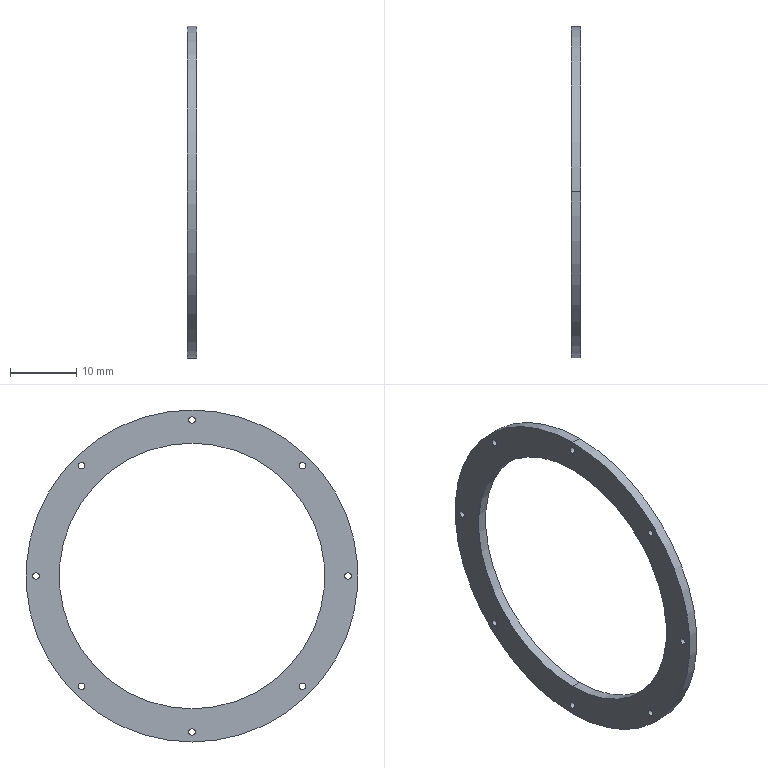Part | SolidWorks | features SavedExtBody 1 | 1 solid | 22 faces | box 1.5 x 50 x 50 mm | volume 1051 mm3 | cylinder 20 | plane 2 | commonest cylinder face diameters 1 x16 40 x2 50 x2
STEP:
#1=CARTESIAN_POINT('',(-88.272,23.5,64.5));
#2=VERTEX_POINT('',#1);
#3=CARTESIAN_POINT('',(-88.272,23.5,65.5));
#4=VERTEX_POINT('',#3);
#5=CARTESIAN_POINT('',(-88.272,23.5,65.));
#6=DIRECTION('',(-1.,0.,0.));
#7=DIRECTION('',(0.,0.,1.));
#8=AXIS2_PLACEMENT_3D('',#5,#6,#7);
#9=CIRCLE('',#8,0.5);
#10=EDGE_CURVE('',#2,#4,#9,.T.);
#11=ORIENTED_EDGE('',*,*,#10,.F.);
#12=CARTESIAN_POINT('',(-89.772,23.5,64.5));
#13=VERTEX_POINT('',#12);
#14=CARTESIAN_POINT('',(-88.272,23.5,64.5));
#15=DIRECTION('',(-1.,0.,0.));
#16=VECTOR('',#15,1000.);
#17=LINE('',#14,#16);
#18=EDGE_CURVE('',#2,#13,#17,.T.);
#19=ORIENTED_EDGE('',*,*,#18,.T.);
#20=CARTESIAN_POINT('',(-89.772,23.5,65.5));
#21=VERTEX_POINT('',#20);
#22=CARTESIAN_POINT('',(-89.772,23.5,65.));
#23=DIRECTION('',(-1.,0.,0.));
#24=DIRECTION('',(0.,0.,1.));
#25=AXIS2_PLACEMENT_3D('',#22,#23,#24);
#26=CIRCLE('',#25,0.5);
#27=EDGE_CURVE('',#13,#21,#26,.T.);
#28=ORIENTED_EDGE('',*,*,#27,.T.);
#29=CARTESIAN_POINT('',(-88.272,23.5,65.5));
#30=DIRECTION('',(-1.,0.,0.));
#31=VECTOR('',#30,1000.);
#32=LINE('',#29,#31);
#33=EDGE_CURVE('',#4,#21,#32,.T.);
#34=ORIENTED_EDGE('',*,*,#33,.F.);
#35=EDGE_LOOP('',(#11,#19,#28,#34));
#36=FACE_OUTER_BOUND('',#35,.T.);
#37=CARTESIAN_POINT('',(-88.272,23.5,65.));
#38=DIRECTION('',(-1.,0.,0.));
#39=DIRECTION('',(0.,0.,1.));
#40=AXIS2_PLACEMENT_3D('',#37,#38,#39);
#41=CYLINDRICAL_SURFACE('',#40,0.5);
#42=ADVANCED_FACE('',(#36),#41,.F.);
#43=CARTESIAN_POINT('',(-88.272,16.617,81.117));
#44=VERTEX_POINT('',#43);
#45=CARTESIAN_POINT('',(-88.272,16.617,82.117));
#46=VERTEX_POINT('',#45);
#47=CARTESIAN_POINT('',(-88.272,16.617,81.617));
#48=DIRECTION('',(-1.,0.,0.));
#49=DIRECTION('',(0.,0.,1.));
#50=AXIS2_PLACEMENT_3D('',#47,#48,#49);
#51=CIRCLE('',#50,0.5);
#52=EDGE_CURVE('',#44,#46,#51,.T.);
#53=ORIENTED_EDGE('',*,*,#52,.F.);
#54=CARTESIAN_POINT('',(-89.772,16.617,81.117));
#55=VERTEX_POINT('',#54);
#56=CARTESIAN_POINT('',(-88.272,16.617,81.117));
#57=DIRECTION('',(-1.,0.,0.));
#58=VECTOR('',#57,1000.);
#59=LINE('',#56,#58);
#60=EDGE_CURVE('',#44,#55,#59,.T.);
#61=ORIENTED_EDGE('',*,*,#60,.T.);
#62=CARTESIAN_POINT('',(-89.772,16.617,82.117));
#63=VERTEX_POINT('',#62);
#64=CARTESIAN_POINT('',(-89.772,16.617,81.617));
#65=DIRECTION('',(-1.,0.,0.));
#66=DIRECTION('',(0.,0.,1.));
#67=AXIS2_PLACEMENT_3D('',#64,#65,#66);
#68=CIRCLE('',#67,0.5);
#69=EDGE_CURVE('',#55,#63,#68,.T.);
#70=ORIENTED_EDGE('',*,*,#69,.T.);
#71=CARTESIAN_POINT('',(-88.272,16.617,82.117));
#72=DIRECTION('',(-1.,0.,0.));
#73=VECTOR('',#72,1000.);
#74=LINE('',#71,#73);
#75=EDGE_CURVE('',#46,#63,#74,.T.);
#76=ORIENTED_EDGE('',*,*,#75,.F.);
#77=EDGE_LOOP('',(#53,#61,#70,#76));
#78=FACE_OUTER_BOUND('',#77,.T.);
#79=CARTESIAN_POINT('',(-88.272,16.617,81.617));
#80=DIRECTION('',(-1.,0.,0.));
#81=DIRECTION('',(0.,0.,1.));
#82=AXIS2_PLACEMENT_3D('',#79,#80,#81);
#83=CYLINDRICAL_SURFACE('',#82,0.5);
#84=ADVANCED_FACE('',(#78),#83,.F.);
#85=CARTESIAN_POINT('',(-88.272,0.,88.));
#86=VERTEX_POINT('',#85);
#87=CARTESIAN_POINT('',(-88.272,0.,89.));
#88=VERTEX_POINT('',#87);
#89=CARTESIAN_POINT('',(-88.272,0.,88.5));
#90=DIRECTION('',(-1.,0.,0.));
#91=DIRECTION('',(0.,0.,1.));
#92=AXIS2_PLACEMENT_3D('',#89,#90,#91);
#93=CIRCLE('',#92,0.5);
#94=EDGE_CURVE('',#86,#88,#93,.T.);
#95=ORIENTED_EDGE('',*,*,#94,.F.);
#96=CARTESIAN_POINT('',(-89.772,0.,88.));
#97=VERTEX_POINT('',#96);
#98=CARTESIAN_POINT('',(-88.272,0.,88.));
#99=DIRECTION('',(-1.,0.,0.));
#100=VECTOR('',#99,1000.);
#101=LINE('',#98,#100);
#102=EDGE_CURVE('',#86,#97,#101,.T.);
#103=ORIENTED_EDGE('',*,*,#102,.T.);
#104=CARTESIAN_POINT('',(-89.772,0.,89.));
#105=VERTEX_POINT('',#104);
#106=CARTESIAN_POINT('',(-89.772,0.,88.5));
#107=DIRECTION('',(-1.,0.,0.));
#108=DIRECTION('',(0.,0.,1.));
#109=AXIS2_PLACEMENT_3D('',#106,#107,#108);
#110=CIRCLE('',#109,0.5);
#111=EDGE_CURVE('',#97,#105,#110,.T.);
#112=ORIENTED_EDGE('',*,*,#111,.T.);
#113=CARTESIAN_POINT('',(-88.272,0.,89.));
#114=DIRECTION('',(-1.,0.,0.));
#115=VECTOR('',#114,1000.);
#116=LINE('',#113,#115);
#117=EDGE_CURVE('',#88,#105,#116,.T.);
#118=ORIENTED_EDGE('',*,*,#117,.F.);
#119=EDGE_LOOP('',(#95,#103,#112,#118));
#120=FACE_OUTER_BOUND('',#119,.T.);
#121=CARTESIAN_POINT('',(-88.272,0.,88.5));
#122=DIRECTION('',(-1.,0.,0.));
#123=DIRECTION('',(0.,0.,1.));
#124=AXIS2_PLACEMENT_3D('',#121,#122,#123);
#125=CYLINDRICAL_SURFACE('',#124,0.5);
#126=ADVANCED_FACE('',(#120),#125,.F.);
#127=CARTESIAN_POINT('',(-88.272,-16.617,81.117));
#128=VERTEX_POINT('',#127);
#129=CARTESIAN_POINT('',(-88.272,-16.617,82.117));
#130=VERTEX_POINT('',#129);
#131=CARTESIAN_POINT('',(-88.272,-16.617,81.617));
#132=DIRECTION('',(-1.,0.,0.));
#133=DIRECTION('',(0.,0.,1.));
#134=AXIS2_PLACEMENT_3D('',#131,#132,#133);
#135=CIRCLE('',#134,0.5);
#136=EDGE_CURVE('',#128,#130,#135,.T.);
#137=ORIENTED_EDGE('',*,*,#136,.F.);
#138=CARTESIAN_POINT('',(-89.772,-16.617,81.117));
#139=VERTEX_POINT('',#138);
#140=CARTESIAN_POINT('',(-88.272,-16.617,81.117));
#141=DIRECTION('',(-1.,0.,0.));
#142=VECTOR('',#141,1000.);
#143=LINE('',#140,#142);
#144=EDGE_CURVE('',#128,#139,#143,.T.);
#145=ORIENTED_EDGE('',*,*,#144,.T.);
#146=CARTESIAN_POINT('',(-89.772,-16.617,82.117));
#147=VERTEX_POINT('',#146);
#148=CARTESIAN_POINT('',(-89.772,-16.617,81.617));
#149=DIRECTION('',(-1.,0.,0.));
#150=DIRECTION('',(0.,0.,1.));
#151=AXIS2_PLACEMENT_3D('',#148,#149,#150);
#152=CIRCLE('',#151,0.5);
#153=EDGE_CURVE('',#139,#147,#152,.T.);
#154=ORIENTED_EDGE('',*,*,#153,.T.);
#155=CARTESIAN_POINT('',(-88.272,-16.617,82.117));
#156=DIRECTION('',(-1.,0.,0.));
#157=VECTOR('',#156,1000.);
#158=LINE('',#155,#157);
#159=EDGE_CURVE('',#130,#147,#158,.T.);
#160=ORIENTED_EDGE('',*,*,#159,.F.);
#161=EDGE_LOOP('',(#137,#145,#154,#160));
#162=FACE_OUTER_BOUND('',#161,.T.);
#163=CARTESIAN_POINT('',(-88.272,-16.617,81.617));
#164=DIRECTION('',(-1.,0.,0.));
#165=DIRECTION('',(0.,0.,1.));
#166=AXIS2_PLACEMENT_3D('',#163,#164,#165);
#167=CYLINDRICAL_SURFACE('',#166,0.5);
#168=ADVANCED_FACE('',(#162),#167,.F.);
#169=CARTESIAN_POINT('',(-88.272,-23.5,64.5));
#170=VERTEX_POINT('',#169);
#171=CARTESIAN_POINT('',(-88.272,-23.5,65.5));
#172=VERTEX_POINT('',#171);
#173=CARTESIAN_POINT('',(-88.272,-23.5,65.));
#174=DIRECTION('',(-1.,0.,0.));
#175=DIRECTION('',(0.,0.,1.));
#176=AXIS2_PLACEMENT_3D('',#173,#174,#175);
#177=CIRCLE('',#176,0.5);
#178=EDGE_CURVE('',#170,#172,#177,.T.);
#179=ORIENTED_EDGE('',*,*,#178,.F.);
#180=CARTESIAN_POINT('',(-89.772,-23.5,64.5));
#181=VERTEX_POINT('',#180);
#182=CARTESIAN_POINT('',(-88.272,-23.5,64.5));
#183=DIRECTION('',(-1.,0.,0.));
#184=VECTOR('',#183,1000.);
#185=LINE('',#182,#184);
#186=EDGE_CURVE('',#170,#181,#185,.T.);
#187=ORIENTED_EDGE('',*,*,#186,.T.);
#188=CARTESIAN_POINT('',(-89.772,-23.5,65.5));
#189=VERTEX_POINT('',#188);
#190=CARTESIAN_POINT('',(-89.772,-23.5,65.));
#191=DIRECTION('',(-1.,0.,0.));
#192=DIRECTION('',(0.,0.,1.));
#193=AXIS2_PLACEMENT_3D('',#190,#191,#192);
#194=CIRCLE('',#193,0.5);
#195=EDGE_CURVE('',#181,#189,#194,.T.);
#196=ORIENTED_EDGE('',*,*,#195,.T.);
#197=CARTESIAN_POINT('',(-88.272,-23.5,65.5));
#198=DIRECTION('',(-1.,0.,0.));
#199=VECTOR('',#198,1000.);
#200=LINE('',#197,#199);
#201=EDGE_CURVE('',#172,#189,#200,.T.);
#202=ORIENTED_EDGE('',*,*,#201,.F.);
#203=EDGE_LOOP('',(#179,#187,#196,#202));
#204=FACE_OUTER_BOUND('',#203,.T.);
#205=CARTESIAN_POINT('',(-88.272,-23.5,65.));
#206=DIRECTION('',(-1.,0.,0.));
#207=DIRECTION('',(0.,0.,1.));
#208=AXIS2_PLACEMENT_3D('',#205,#206,#207);
#209=CYLINDRICAL_SURFACE('',#208,0.5);
#210=ADVANCED_FACE('',(#204),#209,.F.);
#211=CARTESIAN_POINT('',(-88.272,-16.617,47.883));
#212=VERTEX_POINT('',#211);
#213=CARTESIAN_POINT('',(-88.272,-16.617,48.883));
#214=VERTEX_POINT('',#213);
#215=CARTESIAN_POINT('',(-88.272,-16.617,48.383));
#216=DIRECTION('',(-1.,0.,0.));
#217=DIRECTION('',(0.,0.,1.));
#218=AXIS2_PLACEMENT_3D('',#215,#216,#217);
#219=CIRCLE('',#218,0.5);
#220=EDGE_CURVE('',#212,#214,#219,.T.);
#221=ORIENTED_EDGE('',*,*,#220,.F.);
#222=CARTESIAN_POINT('',(-89.772,-16.617,47.883));
#223=VERTEX_POINT('',#222);
#224=CARTESIAN_POINT('',(-88.272,-16.617,47.883));
#225=DIRECTION('',(-1.,0.,0.));
#226=VECTOR('',#225,1000.);
#227=LINE('',#224,#226);
#228=EDGE_CURVE('',#212,#223,#227,.T.);
#229=ORIENTED_EDGE('',*,*,#228,.T.);
#230=CARTESIAN_POINT('',(-89.772,-16.617,48.883));
#231=VERTEX_POINT('',#230);
#232=CARTESIAN_POINT('',(-89.772,-16.617,48.383));
#233=DIRECTION('',(-1.,0.,0.));
#234=DIRECTION('',(0.,0.,1.));
#235=AXIS2_PLACEMENT_3D('',#232,#233,#234);
#236=CIRCLE('',#235,0.5);
#237=EDGE_CURVE('',#223,#231,#236,.T.);
#238=ORIENTED_EDGE('',*,*,#237,.T.);
#239=CARTESIAN_POINT('',(-88.272,-16.617,48.883));
#240=DIRECTION('',(-1.,0.,0.));
#241=VECTOR('',#240,1000.);
#242=LINE('',#239,#241);
#243=EDGE_CURVE('',#214,#231,#242,.T.);
#244=ORIENTED_EDGE('',*,*,#243,.F.);
#245=EDGE_LOOP('',(#221,#229,#238,#244));
#246=FACE_OUTER_BOUND('',#245,.T.);
#247=CARTESIAN_POINT('',(-88.272,-16.617,48.383));
#248=DIRECTION('',(-1.,0.,0.));
#249=DIRECTION('',(0.,0.,1.));
#250=AXIS2_PLACEMENT_3D('',#247,#248,#249);
#251=CYLINDRICAL_SURFACE('',#250,0.5);
#252=ADVANCED_FACE('',(#246),#251,.F.);
#253=CARTESIAN_POINT('',(-88.272,0.,41.));
#254=VERTEX_POINT('',#253);
#255=CARTESIAN_POINT('',(-88.272,0.,42.));
#256=VERTEX_POINT('',#255);
#257=CARTESIAN_POINT('',(-88.272,0.,41.5));
#258=DIRECTION('',(-1.,0.,0.));
#259=DIRECTION('',(0.,0.,1.));
#260=AXIS2_PLACEMENT_3D('',#257,#258,#259);
#261=CIRCLE('',#260,0.5);
#262=EDGE_CURVE('',#254,#256,#261,.T.);
#263=ORIENTED_EDGE('',*,*,#262,.F.);
#264=CARTESIAN_POINT('',(-89.772,0.,41.));
#265=VERTEX_POINT('',#264);
#266=CARTESIAN_POINT('',(-88.272,0.,41.));
#267=DIRECTION('',(-1.,0.,0.));
#268=VECTOR('',#267,1000.);
#269=LINE('',#266,#268);
#270=EDGE_CURVE('',#254,#265,#269,.T.);
#271=ORIENTED_EDGE('',*,*,#270,.T.);
#272=CARTESIAN_POINT('',(-89.772,0.,42.));
#273=VERTEX_POINT('',#272);
#274=CARTESIAN_POINT('',(-89.772,0.,41.5));
#275=DIRECTION('',(-1.,0.,0.));
#276=DIRECTION('',(0.,0.,1.));
#277=AXIS2_PLACEMENT_3D('',#274,#275,#276);
#278=CIRCLE('',#277,0.5);
#279=EDGE_CURVE('',#265,#273,#278,.T.);
#280=ORIENTED_EDGE('',*,*,#279,.T.);
#281=CARTESIAN_POINT('',(-88.272,0.,42.));
#282=DIRECTION('',(-1.,0.,0.));
#283=VECTOR('',#282,1000.);
#284=LINE('',#281,#283);
#285=EDGE_CURVE('',#256,#273,#284,.T.);
#286=ORIENTED_EDGE('',*,*,#285,.F.);
#287=EDGE_LOOP('',(#263,#271,#280,#286));
#288=FACE_OUTER_BOUND('',#287,.T.);
#289=CARTESIAN_POINT('',(-88.272,0.,41.5));
#290=DIRECTION('',(-1.,0.,0.));
#291=DIRECTION('',(0.,0.,1.));
#292=AXIS2_PLACEMENT_3D('',#289,#290,#291);
#293=CYLINDRICAL_SURFACE('',#292,0.5);
#294=ADVANCED_FACE('',(#288),#293,.F.);
#295=CARTESIAN_POINT('',(-88.272,16.617,47.883));
#296=VERTEX_POINT('',#295);
#297=CARTESIAN_POINT('',(-88.272,16.617,48.883));
#298=VERTEX_POINT('',#297);
#299=CARTESIAN_POINT('',(-88.272,16.617,48.383));
#300=DIRECTION('',(-1.,0.,0.));
#301=DIRECTION('',(0.,0.,1.));
#302=AXIS2_PLACEMENT_3D('',#299,#300,#301);
#303=CIRCLE('',#302,0.5);
#304=EDGE_CURVE('',#296,#298,#303,.T.);
#305=ORIENTED_EDGE('',*,*,#304,.F.);
#306=CARTESIAN_POINT('',(-89.772,16.617,47.883));
#307=VERTEX_POINT('',#306);
#308=CARTESIAN_POINT('',(-88.272,16.617,47.883));
#309=DIRECTION('',(-1.,0.,0.));
#310=VECTOR('',#309,1000.);
#311=LINE('',#308,#310);
#312=EDGE_CURVE('',#296,#307,#311,.T.);
#313=ORIENTED_EDGE('',*,*,#312,.T.);
#314=CARTESIAN_POINT('',(-89.772,16.617,48.883));
#315=VERTEX_POINT('',#314);
#316=CARTESIAN_POINT('',(-89.772,16.617,48.383));
#317=DIRECTION('',(-1.,0.,0.));
#318=DIRECTION('',(0.,0.,1.));
#319=AXIS2_PLACEMENT_3D('',#316,#317,#318);
#320=CIRCLE('',#319,0.5);
#321=EDGE_CURVE('',#307,#315,#320,.T.);
#322=ORIENTED_EDGE('',*,*,#321,.T.);
#323=CARTESIAN_POINT('',(-88.272,16.617,48.883));
#324=DIRECTION('',(-1.,0.,0.));
#325=VECTOR('',#324,1000.);
#326=LINE('',#323,#325);
#327=EDGE_CURVE('',#298,#315,#326,.T.);
#328=ORIENTED_EDGE('',*,*,#327,.F.);
#329=EDGE_LOOP('',(#305,#313,#322,#328));
#330=FACE_OUTER_BOUND('',#329,.T.);
#331=CARTESIAN_POINT('',(-88.272,16.617,48.383));
#332=DIRECTION('',(-1.,0.,0.));
#333=DIRECTION('',(0.,0.,1.));
#334=AXIS2_PLACEMENT_3D('',#331,#332,#333);
#335=CYLINDRICAL_SURFACE('',#334,0.5);
#336=ADVANCED_FACE('',(#330),#335,.F.);
#337=CARTESIAN_POINT('',(-89.772,0.,45.));
#338=VERTEX_POINT('',#337);
#339=CARTESIAN_POINT('',(-89.772,0.,85.));
#340=VERTEX_POINT('',#339);
#341=CARTESIAN_POINT('',(-89.772,0.,65.));
#342=DIRECTION('',(-1.,0.,0.));
#343=DIRECTION('',(0.,0.,1.));
#344=AXIS2_PLACEMENT_3D('',#341,#342,#343);
#345=CIRCLE('',#344,20.);
#346=EDGE_CURVE('',#338,#340,#345,.T.);
#347=ORIENTED_EDGE('',*,*,#346,.T.);
#348=CARTESIAN_POINT('',(-88.272,0.,85.));
#349=VERTEX_POINT('',#348);
#350=CARTESIAN_POINT('',(-89.772,0.,85.));
#351=DIRECTION('',(1.,0.,0.));
#352=VECTOR('',#351,1000.);
#353=LINE('',#350,#352);
#354=EDGE_CURVE('',#340,#349,#353,.T.);
#355=ORIENTED_EDGE('',*,*,#354,.T.);
#356=CARTESIAN_POINT('',(-88.272,0.,45.));
#357=VERTEX_POINT('',#356);
#358=CARTESIAN_POINT('',(-88.272,0.,65.));
#359=DIRECTION('',(-1.,0.,0.));
#360=DIRECTION('',(0.,0.,1.));
#361=AXIS2_PLACEMENT_3D('',#358,#359,#360);
#362=CIRCLE('',#361,20.);
#363=EDGE_CURVE('',#357,#349,#362,.T.);
#364=ORIENTED_EDGE('',*,*,#363,.F.);
#365=CARTESIAN_POINT('',(-89.772,0.,45.));
#366=DIRECTION('',(1.,0.,0.));
#367=VECTOR('',#366,1000.);
#368=LINE('',#365,#367);
#369=EDGE_CURVE('',#338,#357,#368,.T.);
#370=ORIENTED_EDGE('',*,*,#369,.F.);
#371=EDGE_LOOP('',(#347,#355,#364,#370));
#372=FACE_OUTER_BOUND('',#371,.T.);
#373=CARTESIAN_POINT('',(-89.772,0.,65.));
#374=DIRECTION('',(1.,0.,0.));
#375=DIRECTION('',(0.,0.,-1.));
#376=AXIS2_PLACEMENT_3D('',#373,#374,#375);
#377=CYLINDRICAL_SURFACE('',#376,20.);
#378=ADVANCED_FACE('',(#372),#377,.F.);
#379=CARTESIAN_POINT('',(-89.772,0.,90.));
#380=VERTEX_POINT('',#379);
#381=CARTESIAN_POINT('',(-89.772,0.,40.));
#382=VERTEX_POINT('',#381);
#383=CARTESIAN_POINT('',(-89.772,0.,65.));
#384=DIRECTION('',(-1.,0.,0.));
#385=DIRECTION('',(0.,0.,1.));
#386=AXIS2_PLACEMENT_3D('',#383,#384,#385);
#387=CIRCLE('',#386,25.);
#388=EDGE_CURVE('',#380,#382,#387,.T.);
#389=ORIENTED_EDGE('',*,*,#388,.F.);
#390=CARTESIAN_POINT('',(-88.272,0.,90.));
#391=VERTEX_POINT('',#390);
#392=CARTESIAN_POINT('',(-89.772,0.,90.));
#393=DIRECTION('',(1.,0.,0.));
#394=VECTOR('',#393,1000.);
#395=LINE('',#392,#394);
#396=EDGE_CURVE('',#380,#391,#395,.T.);
#397=ORIENTED_EDGE('',*,*,#396,.T.);
#398=CARTESIAN_POINT('',(-88.272,0.,40.));
#399=VERTEX_POINT('',#398);
#400=CARTESIAN_POINT('',(-88.272,0.,65.));
#401=DIRECTION('',(-1.,0.,0.));
#402=DIRECTION('',(0.,0.,1.));
#403=AXIS2_PLACEMENT_3D('',#400,#401,#402);
#404=CIRCLE('',#403,25.);
#405=EDGE_CURVE('',#391,#399,#404,.T.);
#406=ORIENTED_EDGE('',*,*,#405,.T.);
#407=CARTESIAN_POINT('',(-89.772,0.,40.));
#408=DIRECTION('',(1.,0.,0.));
#409=VECTOR('',#408,1000.);
#410=LINE('',#407,#409);
#411=EDGE_CURVE('',#382,#399,#410,.T.);
#412=ORIENTED_EDGE('',*,*,#411,.F.);
#413=EDGE_LOOP('',(#389,#397,#406,#412));
#414=FACE_OUTER_BOUND('',#413,.T.);
#415=CARTESIAN_POINT('',(-89.772,0.,65.));
#416=DIRECTION('',(1.,0.,0.));
#417=DIRECTION('',(0.,0.,-1.));
#418=AXIS2_PLACEMENT_3D('',#415,#416,#417);
#419=CYLINDRICAL_SURFACE('',#418,25.);
#420=ADVANCED_FACE('',(#414),#419,.T.);
#421=CARTESIAN_POINT('',(-89.772,23.5,65.));
#422=DIRECTION('',(-1.,0.,0.));
#423=DIRECTION('',(0.,0.,1.));
#424=AXIS2_PLACEMENT_3D('',#421,#422,#423);
#425=CIRCLE('',#424,0.5);
#426=EDGE_CURVE('',#21,#13,#425,.T.);
#427=ORIENTED_EDGE('',*,*,#426,.F.);
#428=ORIENTED_EDGE('',*,*,#27,.F.);
#429=EDGE_LOOP('',(#427,#428));
#430=FACE_BOUND('',#429,.T.);
#431=CARTESIAN_POINT('',(-89.772,16.617,81.617));
#432=DIRECTION('',(-1.,0.,0.));
#433=DIRECTION('',(0.,0.,1.));
#434=AXIS2_PLACEMENT_3D('',#431,#432,#433);
#435=CIRCLE('',#434,0.5);
#436=EDGE_CURVE('',#63,#55,#435,.T.);
#437=ORIENTED_EDGE('',*,*,#436,.F.);
#438=ORIENTED_EDGE('',*,*,#69,.F.);
#439=EDGE_LOOP('',(#437,#438));
#440=FACE_BOUND('',#439,.T.);
#441=CARTESIAN_POINT('',(-89.772,0.,88.5));
#442=DIRECTION('',(-1.,0.,0.));
#443=DIRECTION('',(0.,0.,1.));
#444=AXIS2_PLACEMENT_3D('',#441,#442,#443);
#445=CIRCLE('',#444,0.5);
#446=EDGE_CURVE('',#105,#97,#445,.T.);
#447=ORIENTED_EDGE('',*,*,#446,.F.);
#448=ORIENTED_EDGE('',*,*,#111,.F.);
#449=EDGE_LOOP('',(#447,#448));
#450=FACE_BOUND('',#449,.T.);
#451=CARTESIAN_POINT('',(-89.772,-16.617,81.617));
#452=DIRECTION('',(-1.,0.,0.));
#453=DIRECTION('',(0.,0.,1.));
#454=AXIS2_PLACEMENT_3D('',#451,#452,#453);
#455=CIRCLE('',#454,0.5);
#456=EDGE_CURVE('',#147,#139,#455,.T.);
#457=ORIENTED_EDGE('',*,*,#456,.F.);
#458=ORIENTED_EDGE('',*,*,#153,.F.);
#459=EDGE_LOOP('',(#457,#458));
#460=FACE_BOUND('',#459,.T.);
#461=CARTESIAN_POINT('',(-89.772,-23.5,65.));
#462=DIRECTION('',(-1.,0.,0.));
#463=DIRECTION('',(0.,0.,1.));
#464=AXIS2_PLACEMENT_3D('',#461,#462,#463);
#465=CIRCLE('',#464,0.5);
#466=EDGE_CURVE('',#189,#181,#465,.T.);
#467=ORIENTED_EDGE('',*,*,#466,.F.);
#468=ORIENTED_EDGE('',*,*,#195,.F.);
#469=EDGE_LOOP('',(#467,#468));
#470=FACE_BOUND('',#469,.T.);
#471=CARTESIAN_POINT('',(-89.772,-16.617,48.383));
#472=DIRECTION('',(-1.,0.,0.));
#473=DIRECTION('',(0.,0.,1.));
#474=AXIS2_PLACEMENT_3D('',#471,#472,#473);
#475=CIRCLE('',#474,0.5);
#476=EDGE_CURVE('',#231,#223,#475,.T.);
#477=ORIENTED_EDGE('',*,*,#476,.F.);
#478=ORIENTED_EDGE('',*,*,#237,.F.);
#479=EDGE_LOOP('',(#477,#478));
#480=FACE_BOUND('',#479,.T.);
#481=CARTESIAN_POINT('',(-89.772,0.,41.5));
#482=DIRECTION('',(-1.,0.,0.));
#483=DIRECTION('',(0.,0.,1.));
#484=AXIS2_PLACEMENT_3D('',#481,#482,#483);
#485=CIRCLE('',#484,0.5);
#486=EDGE_CURVE('',#273,#265,#485,.T.);
#487=ORIENTED_EDGE('',*,*,#486,.F.);
#488=ORIENTED_EDGE('',*,*,#279,.F.);
#489=EDGE_LOOP('',(#487,#488));
#490=FACE_BOUND('',#489,.T.);
#491=CARTESIAN_POINT('',(-89.772,16.617,48.383));
#492=DIRECTION('',(-1.,0.,0.));
#493=DIRECTION('',(0.,0.,1.));
#494=AXIS2_PLACEMENT_3D('',#491,#492,#493);
#495=CIRCLE('',#494,0.5);
#496=EDGE_CURVE('',#315,#307,#495,.T.);
#497=ORIENTED_EDGE('',*,*,#496,.F.);
#498=ORIENTED_EDGE('',*,*,#321,.F.);
#499=EDGE_LOOP('',(#497,#498));
#500=FACE_BOUND('',#499,.T.);
#501=CARTESIAN_POINT('',(-89.772,0.,65.));
#502=DIRECTION('',(-1.,0.,0.));
#503=DIRECTION('',(0.,0.,1.));
#504=AXIS2_PLACEMENT_3D('',#501,#502,#503);
#505=CIRCLE('',#504,25.);
#506=EDGE_CURVE('',#382,#380,#505,.T.);
#507=ORIENTED_EDGE('',*,*,#506,.T.);
#508=ORIENTED_EDGE('',*,*,#388,.T.);
#509=EDGE_LOOP('',(#507,#508));
#510=FACE_OUTER_BOUND('',#509,.T.);
#511=ORIENTED_EDGE('',*,*,#346,.F.);
#512=CARTESIAN_POINT('',(-89.772,0.,65.));
#513=DIRECTION('',(-1.,0.,0.));
#514=DIRECTION('',(0.,0.,1.));
#515=AXIS2_PLACEMENT_3D('',#512,#513,#514);
#516=CIRCLE('',#515,20.);
#517=EDGE_CURVE('',#340,#338,#516,.T.);
#518=ORIENTED_EDGE('',*,*,#517,.F.);
#519=EDGE_LOOP('',(#511,#518));
#520=FACE_BOUND('',#519,.T.);
#521=CARTESIAN_POINT('',(-89.772,0.,65.));
#522=DIRECTION('',(-1.,0.,0.));
#523=DIRECTION('',(0.,0.,1.));
#524=AXIS2_PLACEMENT_3D('',#521,#522,#523);
#525=PLANE('',#524);
#526=ADVANCED_FACE('',(#430,#440,#450,#460,#470,#480,#490,#500,#510,#520),#525,.T.);
#527=CARTESIAN_POINT('',(-88.272,23.5,65.));
#528=DIRECTION('',(-1.,0.,0.));
#529=DIRECTION('',(0.,0.,1.));
#530=AXIS2_PLACEMENT_3D('',#527,#528,#529);
#531=CIRCLE('',#530,0.5);
#532=EDGE_CURVE('',#4,#2,#531,.T.);
#533=ORIENTED_EDGE('',*,*,#532,.T.);
#534=ORIENTED_EDGE('',*,*,#10,.T.);
#535=EDGE_LOOP('',(#533,#534));
#536=FACE_BOUND('',#535,.T.);
#537=CARTESIAN_POINT('',(-88.272,16.617,81.617));
#538=DIRECTION('',(-1.,0.,0.));
#539=DIRECTION('',(0.,0.,1.));
#540=AXIS2_PLACEMENT_3D('',#537,#538,#539);
#541=CIRCLE('',#540,0.5);
#542=EDGE_CURVE('',#46,#44,#541,.T.);
#543=ORIENTED_EDGE('',*,*,#542,.T.);
#544=ORIENTED_EDGE('',*,*,#52,.T.);
#545=EDGE_LOOP('',(#543,#544));
#546=FACE_BOUND('',#545,.T.);
#547=CARTESIAN_POINT('',(-88.272,0.,88.5));
#548=DIRECTION('',(-1.,0.,0.));
#549=DIRECTION('',(0.,0.,1.));
#550=AXIS2_PLACEMENT_3D('',#547,#548,#549);
#551=CIRCLE('',#550,0.5);
#552=EDGE_CURVE('',#88,#86,#551,.T.);
#553=ORIENTED_EDGE('',*,*,#552,.T.);
#554=ORIENTED_EDGE('',*,*,#94,.T.);
#555=EDGE_LOOP('',(#553,#554));
#556=FACE_BOUND('',#555,.T.);
#557=CARTESIAN_POINT('',(-88.272,-16.617,81.617));
#558=DIRECTION('',(-1.,0.,0.));
#559=DIRECTION('',(0.,0.,1.));
#560=AXIS2_PLACEMENT_3D('',#557,#558,#559);
#561=CIRCLE('',#560,0.5);
#562=EDGE_CURVE('',#130,#128,#561,.T.);
#563=ORIENTED_EDGE('',*,*,#562,.T.);
#564=ORIENTED_EDGE('',*,*,#136,.T.);
#565=EDGE_LOOP('',(#563,#564));
#566=FACE_BOUND('',#565,.T.);
#567=CARTESIAN_POINT('',(-88.272,-23.5,65.));
#568=DIRECTION('',(-1.,0.,0.));
#569=DIRECTION('',(0.,0.,1.));
#570=AXIS2_PLACEMENT_3D('',#567,#568,#569);
#571=CIRCLE('',#570,0.5);
#572=EDGE_CURVE('',#172,#170,#571,.T.);
#573=ORIENTED_EDGE('',*,*,#572,.T.);
#574=ORIENTED_EDGE('',*,*,#178,.T.);
#575=EDGE_LOOP('',(#573,#574));
#576=FACE_BOUND('',#575,.T.);
#577=CARTESIAN_POINT('',(-88.272,-16.617,48.383));
#578=DIRECTION('',(-1.,0.,0.));
#579=DIRECTION('',(0.,0.,1.));
#580=AXIS2_PLACEMENT_3D('',#577,#578,#579);
#581=CIRCLE('',#580,0.5);
#582=EDGE_CURVE('',#214,#212,#581,.T.);
#583=ORIENTED_EDGE('',*,*,#582,.T.);
#584=ORIENTED_EDGE('',*,*,#220,.T.);
#585=EDGE_LOOP('',(#583,#584));
#586=FACE_BOUND('',#585,.T.);
#587=CARTESIAN_POINT('',(-88.272,0.,41.5));
#588=DIRECTION('',(-1.,0.,0.));
#589=DIRECTION('',(0.,0.,1.));
#590=AXIS2_PLACEMENT_3D('',#587,#588,#589);
#591=CIRCLE('',#590,0.5);
#592=EDGE_CURVE('',#256,#254,#591,.T.);
#593=ORIENTED_EDGE('',*,*,#592,.T.);
#594=ORIENTED_EDGE('',*,*,#262,.T.);
#595=EDGE_LOOP('',(#593,#594));
#596=FACE_BOUND('',#595,.T.);
#597=CARTESIAN_POINT('',(-88.272,16.617,48.383));
#598=DIRECTION('',(-1.,0.,0.));
#599=DIRECTION('',(0.,0.,1.));
#600=AXIS2_PLACEMENT_3D('',#597,#598,#599);
#601=CIRCLE('',#600,0.5);
#602=EDGE_CURVE('',#298,#296,#601,.T.);
#603=ORIENTED_EDGE('',*,*,#602,.T.);
#604=ORIENTED_EDGE('',*,*,#304,.T.);
#605=EDGE_LOOP('',(#603,#604));
#606=FACE_BOUND('',#605,.T.);
#607=CARTESIAN_POINT('',(-88.272,0.,65.));
#608=DIRECTION('',(-1.,0.,0.));
#609=DIRECTION('',(0.,0.,1.));
#610=AXIS2_PLACEMENT_3D('',#607,#608,#609);
#611=CIRCLE('',#610,25.);
#612=EDGE_CURVE('',#399,#391,#611,.T.);
#613=ORIENTED_EDGE('',*,*,#612,.F.);
#614=ORIENTED_EDGE('',*,*,#405,.F.);
#615=EDGE_LOOP('',(#613,#614));
#616=FACE_OUTER_BOUND('',#615,.T.);
#617=ORIENTED_EDGE('',*,*,#363,.T.);
#618=CARTESIAN_POINT('',(-88.272,0.,65.));
#619=DIRECTION('',(-1.,0.,0.));
#620=DIRECTION('',(0.,0.,1.));
#621=AXIS2_PLACEMENT_3D('',#618,#619,#620);
#622=CIRCLE('',#621,20.);
#623=EDGE_CURVE('',#349,#357,#622,.T.);
#624=ORIENTED_EDGE('',*,*,#623,.T.);
#625=EDGE_LOOP('',(#617,#624));
#626=FACE_BOUND('',#625,.T.);
#627=CARTESIAN_POINT('',(-88.272,0.,65.));
#628=DIRECTION('',(-1.,0.,0.));
#629=DIRECTION('',(0.,0.,1.));
#630=AXIS2_PLACEMENT_3D('',#627,#628,#629);
#631=PLANE('',#630);
#632=ADVANCED_FACE('',(#536,#546,#556,#566,#576,#586,#596,#606,#616,#626),#631,.F.);
#633=ORIENTED_EDGE('',*,*,#396,.F.);
#634=ORIENTED_EDGE('',*,*,#506,.F.);
#635=ORIENTED_EDGE('',*,*,#411,.T.);
#636=ORIENTED_EDGE('',*,*,#612,.T.);
#637=EDGE_LOOP('',(#633,#634,#635,#636));
#638=FACE_OUTER_BOUND('',#637,.T.);
#639=CARTESIAN_POINT('',(-89.772,0.,65.));
#640=DIRECTION('',(1.,0.,0.));
#641=DIRECTION('',(0.,0.,-1.));
#642=AXIS2_PLACEMENT_3D('',#639,#640,#641);
#643=CYLINDRICAL_SURFACE('',#642,25.);
#644=ADVANCED_FACE('',(#638),#643,.T.);
#645=ORIENTED_EDGE('',*,*,#354,.F.);
#646=ORIENTED_EDGE('',*,*,#517,.T.);
#647=ORIENTED_EDGE('',*,*,#369,.T.);
#648=ORIENTED_EDGE('',*,*,#623,.F.);
#649=EDGE_LOOP('',(#645,#646,#647,#648));
#650=FACE_OUTER_BOUND('',#649,.T.);
#651=CARTESIAN_POINT('',(-89.772,0.,65.));
#652=DIRECTION('',(1.,0.,0.));
#653=DIRECTION('',(0.,0.,-1.));
#654=AXIS2_PLACEMENT_3D('',#651,#652,#653);
#655=CYLINDRICAL_SURFACE('',#654,20.);
#656=ADVANCED_FACE('',(#650),#655,.F.);
#657=ORIENTED_EDGE('',*,*,#312,.F.);
#658=ORIENTED_EDGE('',*,*,#602,.F.);
#659=ORIENTED_EDGE('',*,*,#327,.T.);
#660=ORIENTED_EDGE('',*,*,#496,.T.);
#661=EDGE_LOOP('',(#657,#658,#659,#660));
#662=FACE_OUTER_BOUND('',#661,.T.);
#663=CARTESIAN_POINT('',(-88.272,16.617,48.383));
#664=DIRECTION('',(-1.,0.,0.));
#665=DIRECTION('',(0.,0.,1.));
#666=AXIS2_PLACEMENT_3D('',#663,#664,#665);
#667=CYLINDRICAL_SURFACE('',#666,0.5);
#668=ADVANCED_FACE('',(#662),#667,.F.);
#669=ORIENTED_EDGE('',*,*,#270,.F.);
#670=ORIENTED_EDGE('',*,*,#592,.F.);
#671=ORIENTED_EDGE('',*,*,#285,.T.);
#672=ORIENTED_EDGE('',*,*,#486,.T.);
#673=EDGE_LOOP('',(#669,#670,#671,#672));
#674=FACE_OUTER_BOUND('',#673,.T.);
#675=CARTESIAN_POINT('',(-88.272,0.,41.5));
#676=DIRECTION('',(-1.,0.,0.));
#677=DIRECTION('',(0.,0.,1.));
#678=AXIS2_PLACEMENT_3D('',#675,#676,#677);
#679=CYLINDRICAL_SURFACE('',#678,0.5);
#680=ADVANCED_FACE('',(#674),#679,.F.);
#681=ORIENTED_EDGE('',*,*,#228,.F.);
#682=ORIENTED_EDGE('',*,*,#582,.F.);
#683=ORIENTED_EDGE('',*,*,#243,.T.);
#684=ORIENTED_EDGE('',*,*,#476,.T.);
#685=EDGE_LOOP('',(#681,#682,#683,#684));
#686=FACE_OUTER_BOUND('',#685,.T.);
#687=CARTESIAN_POINT('',(-88.272,-16.617,48.383));
#688=DIRECTION('',(-1.,0.,0.));
#689=DIRECTION('',(0.,0.,1.));
#690=AXIS2_PLACEMENT_3D('',#687,#688,#689);
#691=CYLINDRICAL_SURFACE('',#690,0.5);
#692=ADVANCED_FACE('',(#686),#691,.F.);
#693=ORIENTED_EDGE('',*,*,#186,.F.);
#694=ORIENTED_EDGE('',*,*,#572,.F.);
#695=ORIENTED_EDGE('',*,*,#201,.T.);
#696=ORIENTED_EDGE('',*,*,#466,.T.);
#697=EDGE_LOOP('',(#693,#694,#695,#696));
#698=FACE_OUTER_BOUND('',#697,.T.);
#699=CARTESIAN_POINT('',(-88.272,-23.5,65.));
#700=DIRECTION('',(-1.,0.,0.));
#701=DIRECTION('',(0.,0.,1.));
#702=AXIS2_PLACEMENT_3D('',#699,#700,#701);
#703=CYLINDRICAL_SURFACE('',#702,0.5);
#704=ADVANCED_FACE('',(#698),#703,.F.);
#705=ORIENTED_EDGE('',*,*,#144,.F.);
#706=ORIENTED_EDGE('',*,*,#562,.F.);
#707=ORIENTED_EDGE('',*,*,#159,.T.);
#708=ORIENTED_EDGE('',*,*,#456,.T.);
#709=EDGE_LOOP('',(#705,#706,#707,#708));
#710=FACE_OUTER_BOUND('',#709,.T.);
#711=CARTESIAN_POINT('',(-88.272,-16.617,81.617));
#712=DIRECTION('',(-1.,0.,0.));
#713=DIRECTION('',(0.,0.,1.));
#714=AXIS2_PLACEMENT_3D('',#711,#712,#713);
#715=CYLINDRICAL_SURFACE('',#714,0.5);
#716=ADVANCED_FACE('',(#710),#715,.F.);
#717=ORIENTED_EDGE('',*,*,#102,.F.);
#718=ORIENTED_EDGE('',*,*,#552,.F.);
#719=ORIENTED_EDGE('',*,*,#117,.T.);
#720=ORIENTED_EDGE('',*,*,#446,.T.);
#721=EDGE_LOOP('',(#717,#718,#719,#720));
#722=FACE_OUTER_BOUND('',#721,.T.);
#723=CARTESIAN_POINT('',(-88.272,0.,88.5));
#724=DIRECTION('',(-1.,0.,0.));
#725=DIRECTION('',(0.,0.,1.));
#726=AXIS2_PLACEMENT_3D('',#723,#724,#725);
#727=CYLINDRICAL_SURFACE('',#726,0.5);
#728=ADVANCED_FACE('',(#722),#727,.F.);
#729=ORIENTED_EDGE('',*,*,#60,.F.);
#730=ORIENTED_EDGE('',*,*,#542,.F.);
#731=ORIENTED_EDGE('',*,*,#75,.T.);
#732=ORIENTED_EDGE('',*,*,#436,.T.);
#733=EDGE_LOOP('',(#729,#730,#731,#732));
#734=FACE_OUTER_BOUND('',#733,.T.);
#735=CARTESIAN_POINT('',(-88.272,16.617,81.617));
#736=DIRECTION('',(-1.,0.,0.));
#737=DIRECTION('',(0.,0.,1.));
#738=AXIS2_PLACEMENT_3D('',#735,#736,#737);
#739=CYLINDRICAL_SURFACE('',#738,0.5);
#740=ADVANCED_FACE('',(#734),#739,.F.);
#741=ORIENTED_EDGE('',*,*,#18,.F.);
#742=ORIENTED_EDGE('',*,*,#532,.F.);
#743=ORIENTED_EDGE('',*,*,#33,.T.);
#744=ORIENTED_EDGE('',*,*,#426,.T.);
#745=EDGE_LOOP('',(#741,#742,#743,#744));
#746=FACE_OUTER_BOUND('',#745,.T.);
#747=CARTESIAN_POINT('',(-88.272,23.5,65.));
#748=DIRECTION('',(-1.,0.,0.));
#749=DIRECTION('',(0.,0.,1.));
#750=AXIS2_PLACEMENT_3D('',#747,#748,#749);
#751=CYLINDRICAL_SURFACE('',#750,0.5);
#752=ADVANCED_FACE('',(#746),#751,.F.);
#753=CLOSED_SHELL('',(#42,#84,#126,#168,#210,#252,#294,#336,#378,#420,#526,#632,#644,#656,#668,#680,#692,#704,#716,#728,#740,#752));
#754=MANIFOLD_SOLID_BREP('',#753);
#755=CARTESIAN_POINT('',(0.,0.,0.));
#756=DIRECTION('',(0.,0.,1.));
#757=DIRECTION('',(1.,0.,0.));
#758=AXIS2_PLACEMENT_3D('',#755,#756,#757);
#759=(LENGTH_UNIT()NAMED_UNIT(*)SI_UNIT(.MILLI.,.METRE.));
#760=UNCERTAINTY_MEASURE_WITH_UNIT(LENGTH_MEASURE(0.00001),#759,'','');
#761=(NAMED_UNIT(*)PLANE_ANGLE_UNIT()SI_UNIT($,.RADIAN.));
#762=(NAMED_UNIT(*)SI_UNIT($,.STERADIAN.)SOLID_ANGLE_UNIT());
#763=(GEOMETRIC_REPRESENTATION_CONTEXT(3)GLOBAL_UNCERTAINTY_ASSIGNED_CONTEXT((#760))GLOBAL_UNIT_ASSIGNED_CONTEXT((#759,#761,#762))REPRESENTATION_CONTEXT('',''));
#764=ADVANCED_BREP_SHAPE_REPRESENTATION('',(#754,#758),#763);